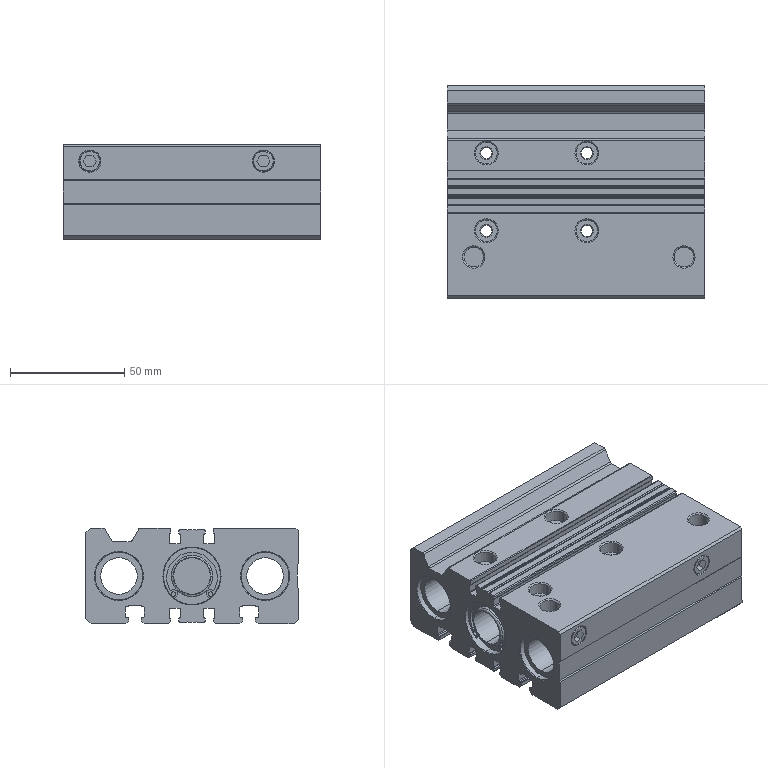Part | SolidWorks | features BaseBody 1 | 1 solid | 390 faces | box 112.5 x 93 x 42 mm | volume 290420 mm3 | cylinder 178 | plane 146 | cone 62 | spline 4 | commonest cylinder face diameters 0.4 x34 0.8 x28 4.917 x16 2 x12 4 x12 1.5 x11